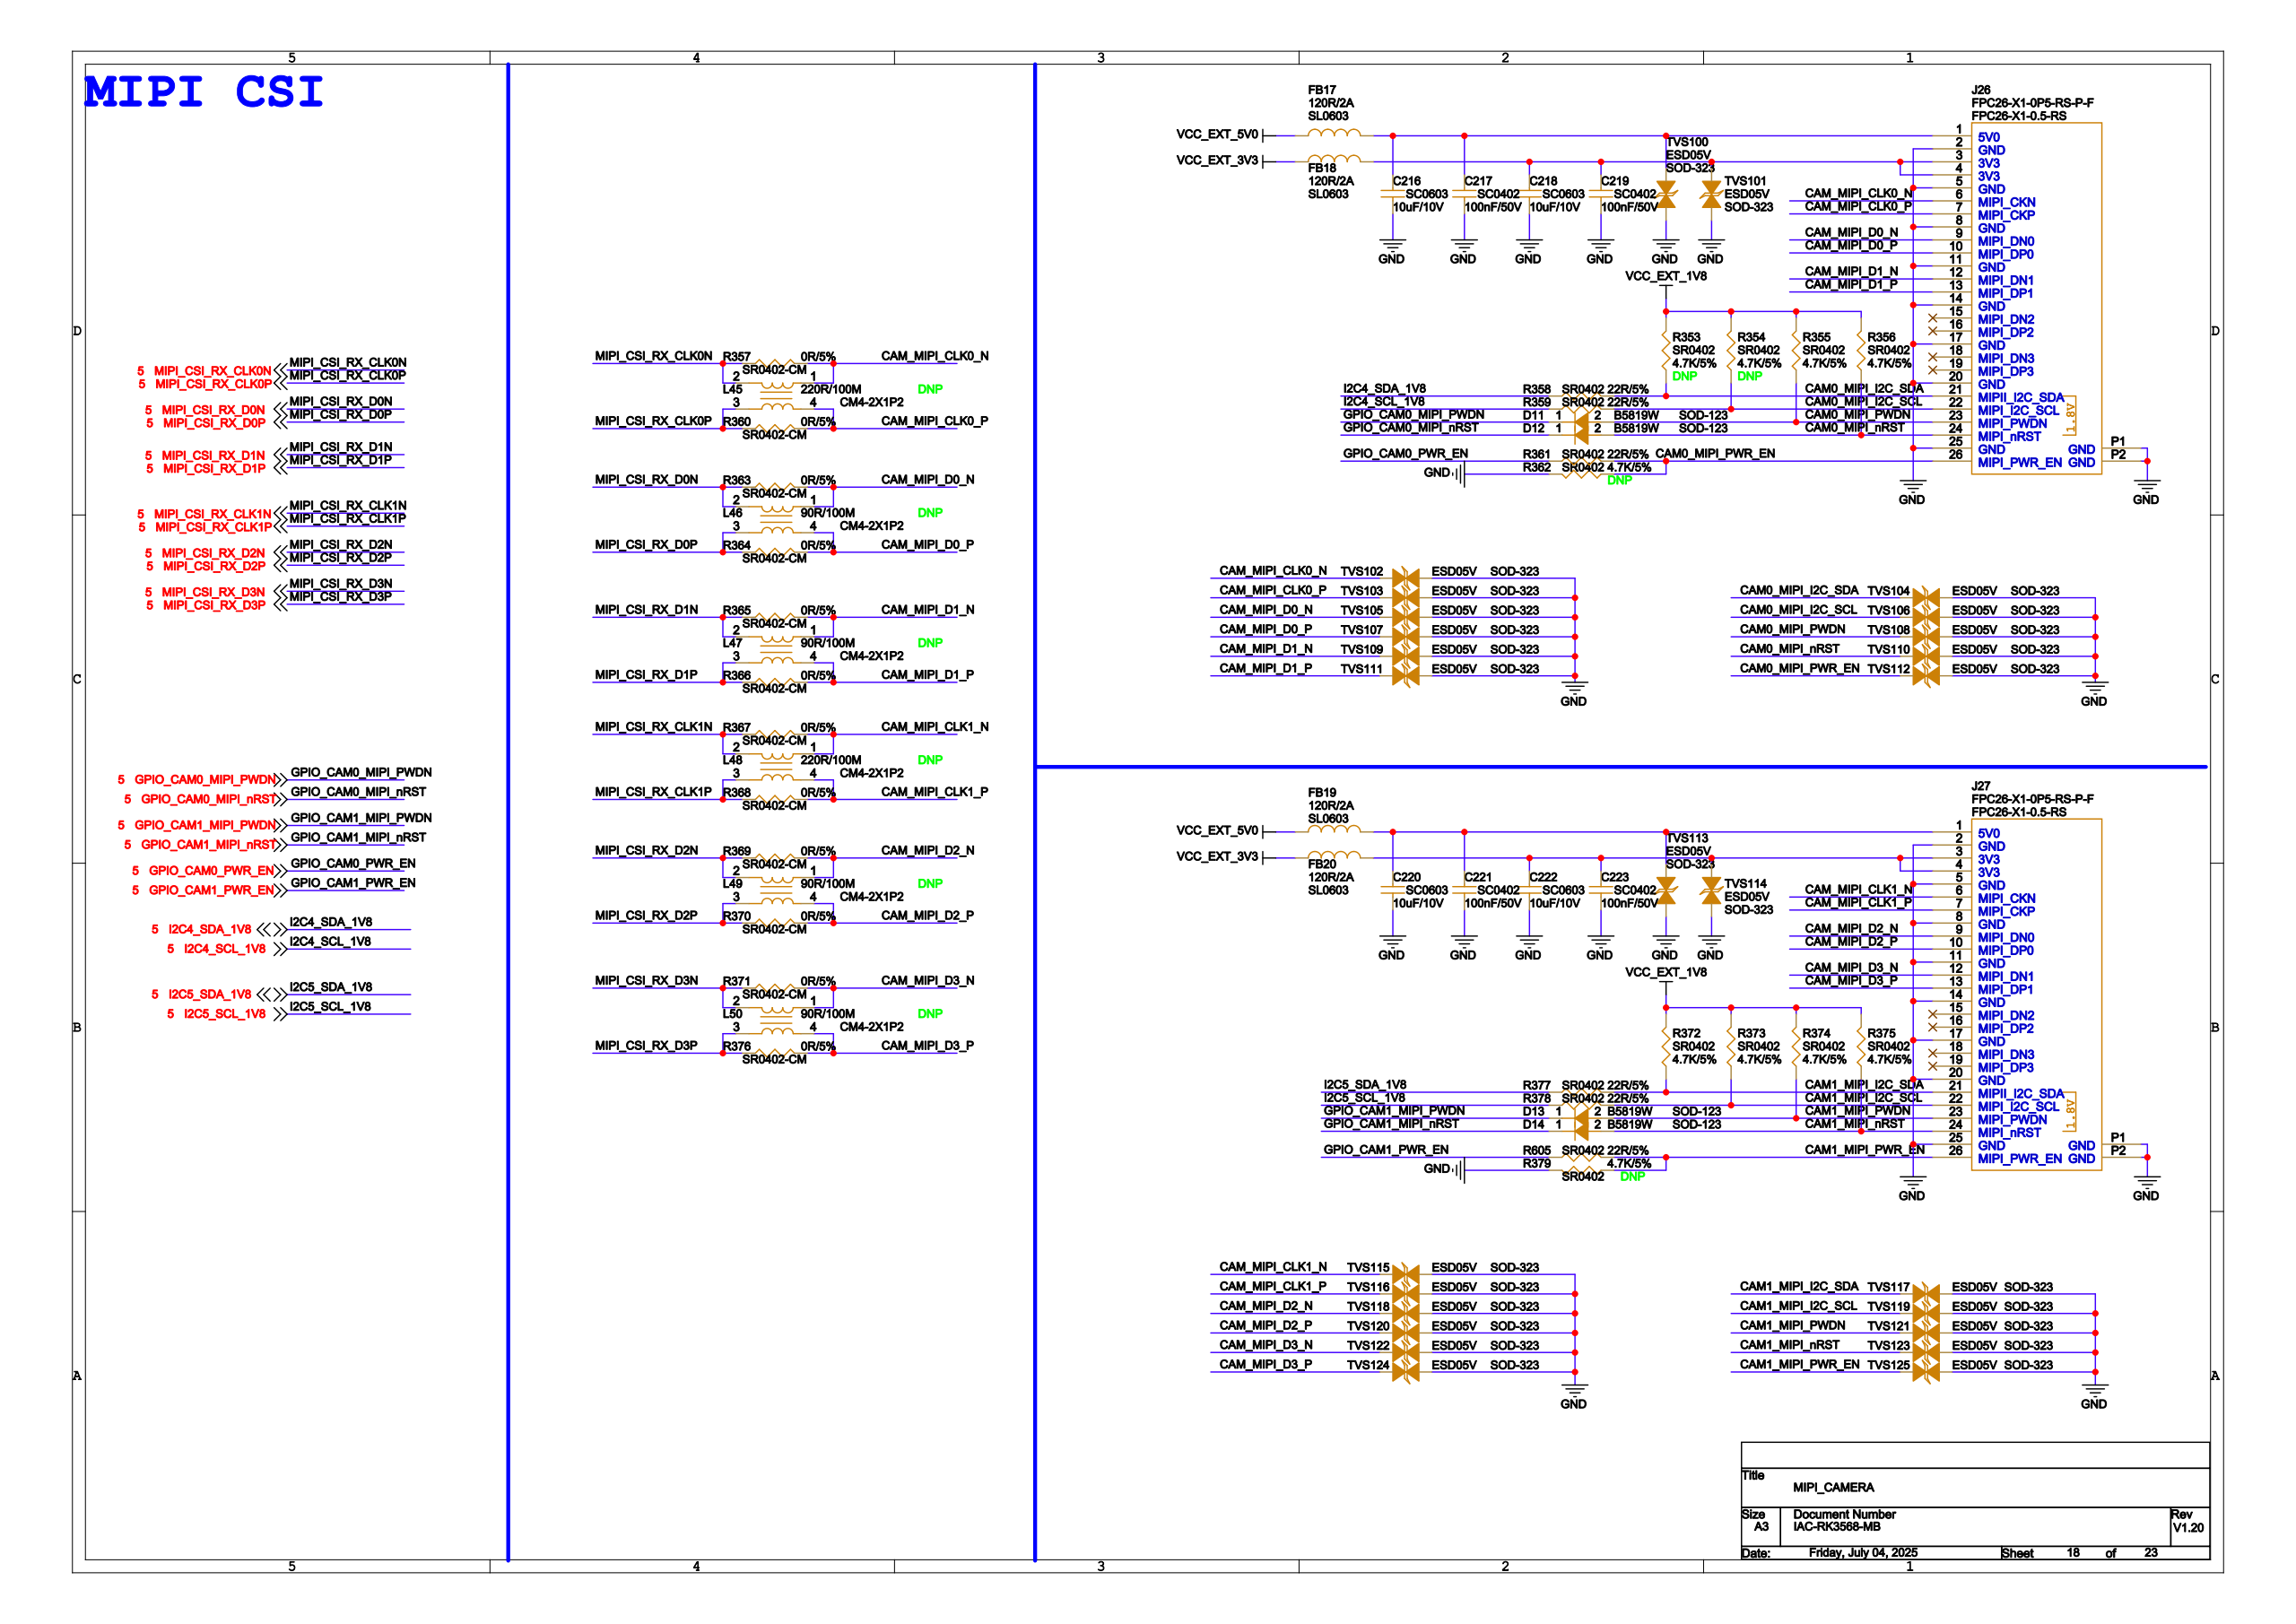Circuit board | Cadence Allegro | 1138 parts | 722 nets | one sheet of the schematic
Parts on this sheet (reference | value | footprint):
C216 | 10uF/10V | SC0603
C217 | 100nF/50V | SC0402
C218 | 10uF/10V | SC0603
C219 | 100nF/50V | SC0402
C220 | 10uF/10V | SC0603
C221 | 100nF/50V | SC0402
C222 | 10uF/10V | SC0603
C223 | 100nF/50V | SC0402
D11 | B5819W | SOD-123
D12 | B5819W | SOD-123
D13 | B5819W | SOD-123
D14 | B5819W | SOD-123
FB17 | 120R/2A | SL0603
FB18 | 120R/2A | SL0603
FB19 | 120R/2A | SL0603
FB20 | 120R/2A | SL0603
J26 | FPC26-X1-0.5-RS | FPC26-X1-0P5-RS-P-F
J27 | FPC26-X1-0.5-RS | FPC26-X1-0P5-RS-P-F
L45 | 220R/100M | CM4-2X1P2
L46 | 90R/100M | CM4-2X1P2
L47 | 90R/100M | CM4-2X1P2
L48 | 220R/100M | CM4-2X1P2
L49 | 90R/100M | CM4-2X1P2
L50 | 90R/100M | CM4-2X1P2
R353 | 4.7K/5% | SR0402
R354 | 4.7K/5% | SR0402
R355 | 4.7K/5% | SR0402
R356 | 4.7K/5% | SR0402
R357 | 0R/5% | SR0402-CM
R358 | 22R/5% | SR0402
R359 | 22R/5% | SR0402
R360 | 0R/5% | SR0402-CM
R361 | 22R/5% | SR0402
R362 | 4.7K/5% | SR0402
R363 | 0R/5% | SR0402-CM
R364 | 0R/5% | SR0402-CM
R365 | 0R/5% | SR0402-CM
R366 | 0R/5% | SR0402-CM
R367 | 0R/5% | SR0402-CM
R368 | 0R/5% | SR0402-CM
R369 | 0R/5% | SR0402-CM
R370 | 0R/5% | SR0402-CM
R371 | 0R/5% | SR0402-CM
R372 | 4.7K/5% | SR0402
R373 | 4.7K/5% | SR0402
R374 | 4.7K/5% | SR0402
R375 | 4.7K/5% | SR0402
R376 | 0R/5% | SR0402-CM
R377 | 22R/5% | SR0402
R378 | 22R/5% | SR0402
R379 | 4.7K/5% | SR0402
R605 | 22R/5% | SR0402
TVS100 | ESD05V | SOD-323
TVS101 | ESD05V | SOD-323
TVS102 | ESD05V | SOD-323
TVS103 | ESD05V | SOD-323
TVS104 | ESD05V | SOD-323
TVS105 | ESD05V | SOD-323
TVS106 | ESD05V | SOD-323
TVS107 | ESD05V | SOD-323
TVS108 | ESD05V | SOD-323
TVS109 | ESD05V | SOD-323
TVS110 | ESD05V | SOD-323
TVS111 | ESD05V | SOD-323
TVS112 | ESD05V | SOD-323
TVS113 | ESD05V | SOD-323
TVS114 | ESD05V | SOD-323
TVS115 | ESD05V | SOD-323
TVS116 | ESD05V | SOD-323
TVS117 | ESD05V | SOD-323
TVS118 | ESD05V | SOD-323
TVS119 | ESD05V | SOD-323
TVS120 | ESD05V | SOD-323
TVS121 | ESD05V | SOD-323
TVS122 | ESD05V | SOD-323
TVS123 | ESD05V | SOD-323
TVS124 | ESD05V | SOD-323
TVS125 | ESD05V | SOD-323
Nets of these parts (net: part-pin ...):
CAM0_MIPI_PWDN: D11-2 R355-1 TVS108-1 J26-23
GPIO_CAM0_MIPI_PWDN: D11-1
CAM0_MIPI_NRST: D12-2 R356-1 TVS110-1 J26-24
GPIO_CAM0_MIPI_NRST: D12-1
CAM1_MIPI_PWDN: D13-2 R374-1 TVS121-1 J27-23
GPIO_CAM1_MIPI_PWDN: D13-1
CAM1_MIPI_NRST: D14-2 R375-1 TVS123-1 J27-24
GPIO_CAM1_MIPI_NRST: D14-1
VCC_EXT_5V0: FB17-1 FB19-1
VCC_EXT_3V3: FB18-1 FB20-1
GND: C216-2 C217-2 C218-2 C219-2 C220-2 C221-2 C222-2 C223-2 R362-2 R379-2 TVS100-1 TVS101-1 TVS102-2 TVS103-2 TVS104-2 TVS105-2 TVS106-2 TVS107-2 TVS108-2 TVS109-2 TVS110-2 TVS111-2 TVS112-2 TVS113-1 TVS114-1 TVS115-2 TVS116-2 TVS117-2 TVS118-2 TVS119-2 TVS120-2 TVS121-2 TVS122-2 TVS123-2 TVS124-2 TVS125-2 J26-2 J26-5 J26-8 J26-11 J26-14 J26-17 J26-20 J26-25 J26-P1 J26-P2 J27-2 J27-5 J27-8 J27-11 J27-14 J27-17 J27-20 J27-25 J27-P1 J27-P2
N19599010: C216-1 C217-1 FB17-2 TVS100-2 J26-1
N19599028: C218-1 C219-1 FB18-2 TVS101-2 J26-3 J26-4
CAM_MIPI_CLK0_N: L45-1 R357-2 TVS102-1 J26-6
CAM_MIPI_CLK0_P: L45-4 R360-2 TVS103-1 J26-7
CAM0_MIPI_I2C_SDA: R353-1 R358-2 TVS104-1 J26-21
CAM_MIPI_D0_N: L46-1 R363-2 TVS105-1 J26-9
CAM0_MIPI_I2C_SCL: R354-1 R359-2 TVS106-1 J26-22
CAM_MIPI_D0_P: L46-4 R364-2 TVS107-1 J26-10
CAM_MIPI_D1_N: L47-1 R365-2 TVS109-1 J26-12
CAM_MIPI_D1_P: L47-4 R366-2 TVS111-1 J26-13
CAM0_MIPI_PWR_EN: R361-2 R362-1 TVS112-1 J26-26
N3943034: C220-1 C221-1 FB19-2 TVS113-2 J27-1
N3943058: C222-1 C223-1 FB20-2 TVS114-2 J27-3 J27-4
CAM_MIPI_CLK1_N: L48-1 R367-2 TVS115-1 J27-6
CAM_MIPI_CLK1_P: L48-4 R368-2 TVS116-1 J27-7
CAM1_MIPI_I2C_SDA: R372-1 R377-2 TVS117-1 J27-21
CAM_MIPI_D2_N: L49-1 R369-2 TVS118-1 J27-9
CAM1_MIPI_I2C_SCL: R373-1 R378-2 TVS119-1 J27-22
CAM_MIPI_D2_P: L49-4 R370-2 TVS120-1 J27-10
CAM_MIPI_D3_N: L50-1 R371-2 TVS122-1 J27-12
CAM_MIPI_D3_P: L50-4 R376-2 TVS124-1 J27-13
CAM1_MIPI_PWR_EN: R379-1 R605-2 TVS125-1 J27-26
MIPI_CSI_RX_CLK0N: L45-2 R357-1
MIPI_CSI_RX_CLK0P: L45-3 R360-1
MIPI_CSI_RX_CLK1N: L48-2 R367-1
MIPI_CSI_RX_CLK1P: L48-3 R368-1
MIPI_CSI_RX_D0N: L46-2 R363-1
MIPI_CSI_RX_D0P: L46-3 R364-1
MIPI_CSI_RX_D1N: L47-2 R365-1
MIPI_CSI_RX_D1P: L47-3 R366-1
MIPI_CSI_RX_D2N: L49-2 R369-1
MIPI_CSI_RX_D2P: L49-3 R370-1
MIPI_CSI_RX_D3N: L50-2 R371-1
MIPI_CSI_RX_D3P: L50-3 R376-1
VCC_EXT_1V8: R353-2 R354-2 R355-2 R356-2 R372-2 R373-2 R374-2 R375-2
GPIO_CAM0_PWR_EN: R361-1
GPIO_CAM1_PWR_EN: R605-1
I2C4_SDA_1V8: R358-1
I2C4_SCL_1V8: R359-1
I2C5_SDA_1V8: R377-1
I2C5_SCL_1V8: R378-1